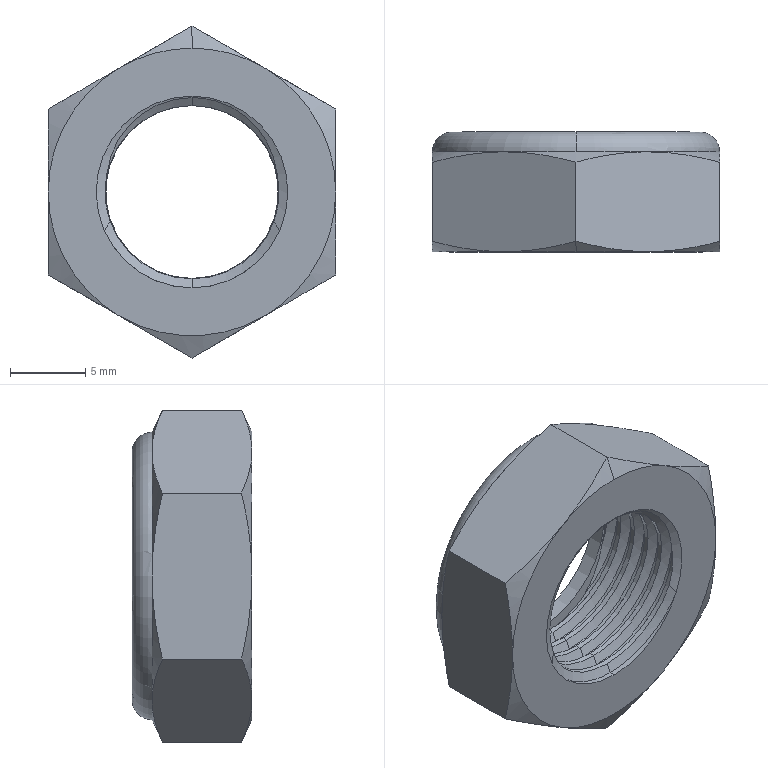Part | SolidWorks | features RevCut 4, Revolution 2, CombineBodies 1, Extrusion 1, LPattern 1 | 2 solids | 84 faces | box 19.05 x 7.938 x 21.997 mm | volume 1490 mm3 | cone 38 | cylinder 28 | plane 12 | torus 6 | commonest cylinder face diameters 12.7 x13 11.531 x11 11.443 x2 13.923 x2